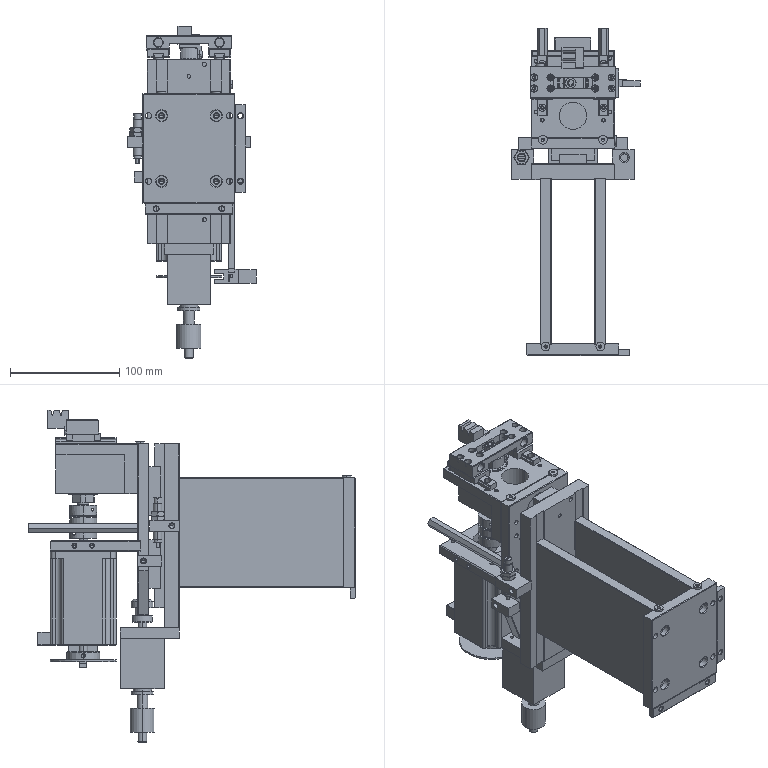Part | NX | 50 solids | 2395 faces | box 117.6 x 298.9 x 303.5 mm | volume 1392568 mm3 | plane 1260 | cylinder 688 | cone 401 | torus 40 | sphere 4 | spline 2 | commonest cylinder face diameters 2.5 x86 8 x69 4.2 x48 5.5 x44 6 x43 3.3 x40